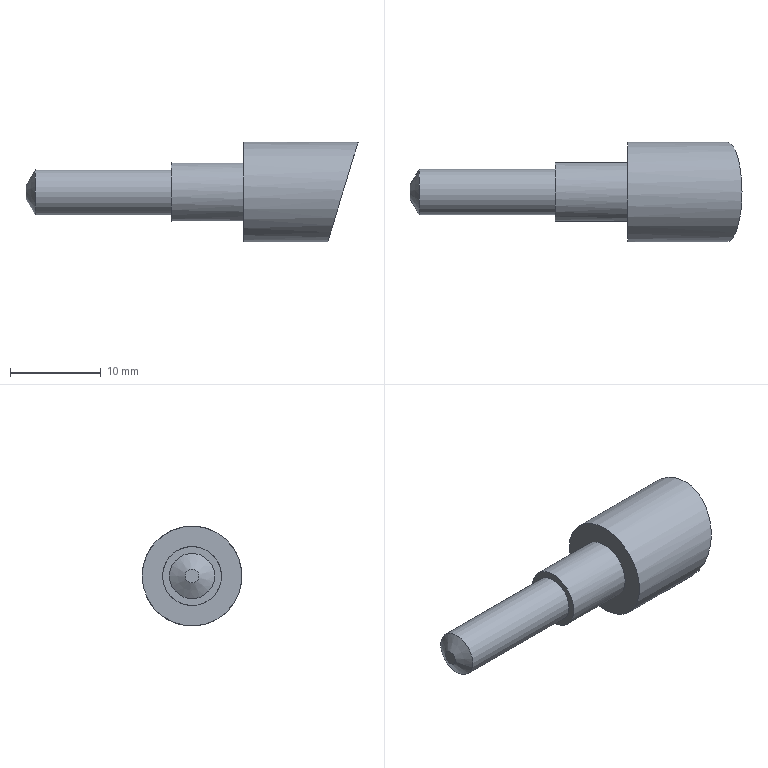Part | STEP file | solid 153 | 1 solid | 8 faces | box 36.597 x 11 x 11 mm | volume 1608 mm3 | plane 4 | cylinder 3 | cone 1 | commonest cylinder face diameters 5 x1 6.5 x1 11 x1